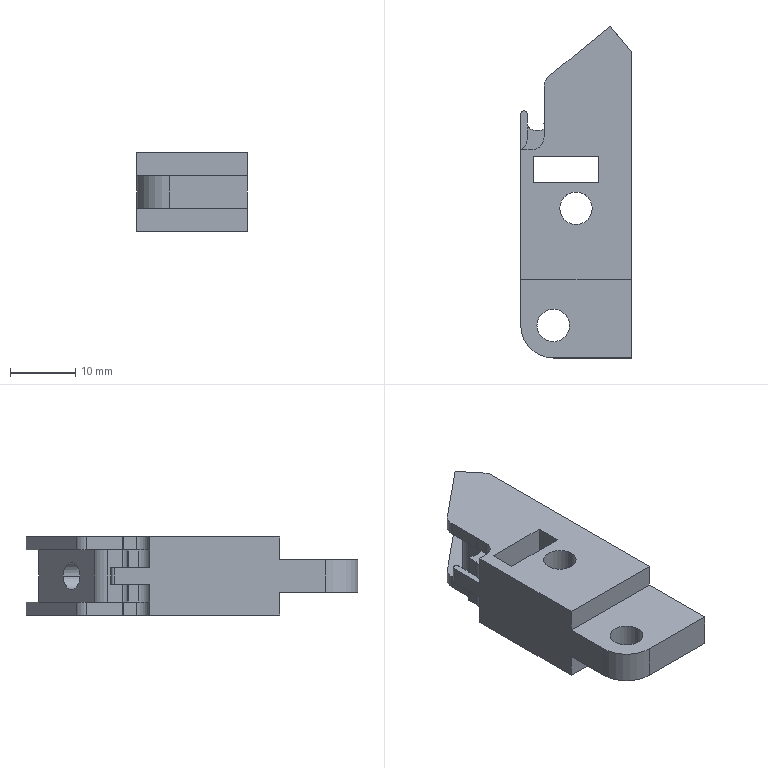Part | STEP file | X77b-01002 | 1 solid | 65 faces | box 17 x 51.049 x 12 mm | volume 6240 mm3 | plane 37 | cylinder 26 | cone 2 | commonest cylinder face diameters 4 x6 5 x4 0.4 x2 1 x2 1.4 x2 2.4 x2